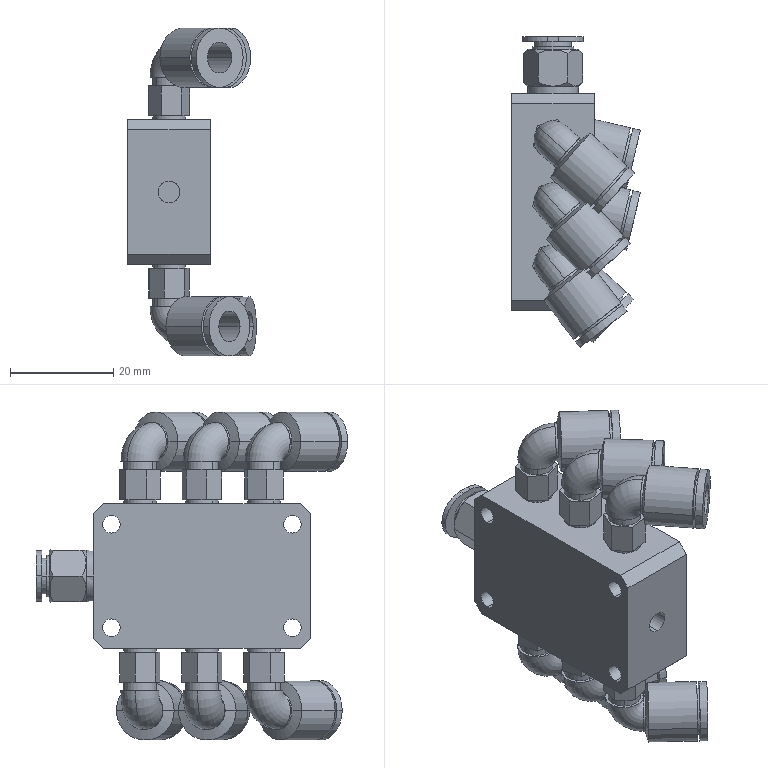Part | SolidWorks | features BaseBody 8 | 8 solids | 339 faces | box 24.892 x 60.174 x 63.5 mm | volume 25312 mm3 | cylinder 143 | plane 133 | cone 51 | torus 12 | commonest cylinder face diameters 6.3 x24 11.5 x24 6 x22 4.2 x19 5 x12 7.36 x12